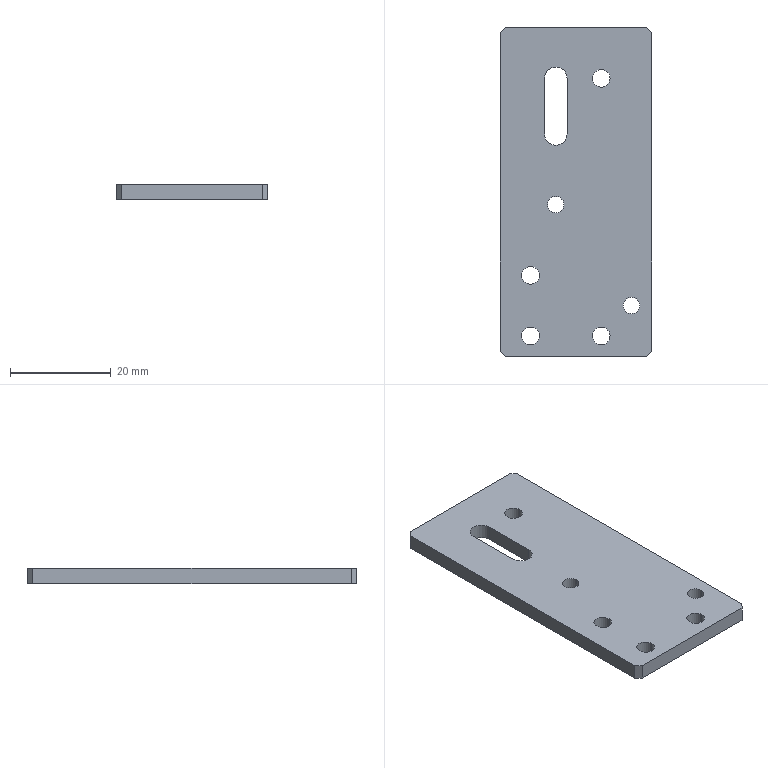Part | SolidWorks | features BaseBody 1 | 1 solid | 26 faces | box 30 x 65 x 3 mm | volume 5483 mm3 | cylinder 14 | plane 12 | commonest cylinder face diameters 3.5 x8 3.242 x4 4.5 x2
STEP:
#1=CARTESIAN_POINT('',(-39.084,79.458,0.));
#2=VERTEX_POINT('',#1);
#3=CARTESIAN_POINT('',(-42.584,79.458,0.));
#4=VERTEX_POINT('',#3);
#5=CARTESIAN_POINT('',(-40.834,79.458,0.));
#6=DIRECTION('',(0.,0.,-1.));
#7=DIRECTION('',(1.,0.,0.));
#8=AXIS2_PLACEMENT_3D('',#5,#6,#7);
#9=CIRCLE('',#8,1.75);
#10=EDGE_CURVE('',#2,#4,#9,.T.);
#11=ORIENTED_EDGE('',*,*,#10,.T.);
#12=CARTESIAN_POINT('',(-42.584,79.458,3.));
#13=VERTEX_POINT('',#12);
#14=CARTESIAN_POINT('',(-42.584,79.458,-68.652));
#15=DIRECTION('',(0.,0.,1.));
#16=VECTOR('',#15,1000.);
#17=LINE('',#14,#16);
#18=EDGE_CURVE('',#4,#13,#17,.T.);
#19=ORIENTED_EDGE('',*,*,#18,.T.);
#20=CARTESIAN_POINT('',(-39.084,79.458,3.));
#21=VERTEX_POINT('',#20);
#22=CARTESIAN_POINT('',(-40.834,79.458,3.));
#23=DIRECTION('',(0.,0.,-1.));
#24=DIRECTION('',(1.,0.,0.));
#25=AXIS2_PLACEMENT_3D('',#22,#23,#24);
#26=CIRCLE('',#25,1.75);
#27=EDGE_CURVE('',#21,#13,#26,.T.);
#28=ORIENTED_EDGE('',*,*,#27,.F.);
#29=CARTESIAN_POINT('',(-39.084,79.458,-68.652));
#30=DIRECTION('',(0.,0.,1.));
#31=VECTOR('',#30,1000.);
#32=LINE('',#29,#31);
#33=EDGE_CURVE('',#2,#21,#32,.T.);
#34=ORIENTED_EDGE('',*,*,#33,.F.);
#35=EDGE_LOOP('',(#11,#19,#28,#34));
#36=FACE_OUTER_BOUND('',#35,.T.);
#37=CARTESIAN_POINT('',(-40.834,79.458,-68.652));
#38=DIRECTION('',(0.,0.,1.));
#39=DIRECTION('',(1.,0.,0.));
#40=AXIS2_PLACEMENT_3D('',#37,#38,#39);
#41=CYLINDRICAL_SURFACE('',#40,1.75);
#42=ADVANCED_FACE('',(#36),#41,.F.);
#43=CARTESIAN_POINT('',(-53.084,79.458,0.));
#44=VERTEX_POINT('',#43);
#45=CARTESIAN_POINT('',(-56.584,79.458,0.));
#46=VERTEX_POINT('',#45);
#47=CARTESIAN_POINT('',(-54.834,79.458,0.));
#48=DIRECTION('',(0.,0.,-1.));
#49=DIRECTION('',(1.,0.,0.));
#50=AXIS2_PLACEMENT_3D('',#47,#48,#49);
#51=CIRCLE('',#50,1.75);
#52=EDGE_CURVE('',#44,#46,#51,.T.);
#53=ORIENTED_EDGE('',*,*,#52,.T.);
#54=CARTESIAN_POINT('',(-56.584,79.458,3.));
#55=VERTEX_POINT('',#54);
#56=CARTESIAN_POINT('',(-56.584,79.458,-68.652));
#57=DIRECTION('',(0.,0.,1.));
#58=VECTOR('',#57,1000.);
#59=LINE('',#56,#58);
#60=EDGE_CURVE('',#46,#55,#59,.T.);
#61=ORIENTED_EDGE('',*,*,#60,.T.);
#62=CARTESIAN_POINT('',(-53.084,79.458,3.));
#63=VERTEX_POINT('',#62);
#64=CARTESIAN_POINT('',(-54.834,79.458,3.));
#65=DIRECTION('',(0.,0.,-1.));
#66=DIRECTION('',(1.,0.,0.));
#67=AXIS2_PLACEMENT_3D('',#64,#65,#66);
#68=CIRCLE('',#67,1.75);
#69=EDGE_CURVE('',#63,#55,#68,.T.);
#70=ORIENTED_EDGE('',*,*,#69,.F.);
#71=CARTESIAN_POINT('',(-53.084,79.458,-68.652));
#72=DIRECTION('',(0.,0.,1.));
#73=VECTOR('',#72,1000.);
#74=LINE('',#71,#73);
#75=EDGE_CURVE('',#44,#63,#74,.T.);
#76=ORIENTED_EDGE('',*,*,#75,.F.);
#77=EDGE_LOOP('',(#53,#61,#70,#76));
#78=FACE_OUTER_BOUND('',#77,.T.);
#79=CARTESIAN_POINT('',(-54.834,79.458,-68.652));
#80=DIRECTION('',(0.,0.,1.));
#81=DIRECTION('',(1.,0.,0.));
#82=AXIS2_PLACEMENT_3D('',#79,#80,#81);
#83=CYLINDRICAL_SURFACE('',#82,1.75);
#84=ADVANCED_FACE('',(#78),#83,.F.);
#85=CARTESIAN_POINT('',(-53.084,91.458,0.));
#86=VERTEX_POINT('',#85);
#87=CARTESIAN_POINT('',(-56.584,91.458,0.));
#88=VERTEX_POINT('',#87);
#89=CARTESIAN_POINT('',(-54.834,91.458,0.));
#90=DIRECTION('',(0.,0.,-1.));
#91=DIRECTION('',(1.,0.,0.));
#92=AXIS2_PLACEMENT_3D('',#89,#90,#91);
#93=CIRCLE('',#92,1.75);
#94=EDGE_CURVE('',#86,#88,#93,.T.);
#95=ORIENTED_EDGE('',*,*,#94,.T.);
#96=CARTESIAN_POINT('',(-56.584,91.458,3.));
#97=VERTEX_POINT('',#96);
#98=CARTESIAN_POINT('',(-56.584,91.458,-68.652));
#99=DIRECTION('',(0.,0.,1.));
#100=VECTOR('',#99,1000.);
#101=LINE('',#98,#100);
#102=EDGE_CURVE('',#88,#97,#101,.T.);
#103=ORIENTED_EDGE('',*,*,#102,.T.);
#104=CARTESIAN_POINT('',(-53.084,91.458,3.));
#105=VERTEX_POINT('',#104);
#106=CARTESIAN_POINT('',(-54.834,91.458,3.));
#107=DIRECTION('',(0.,0.,-1.));
#108=DIRECTION('',(1.,0.,0.));
#109=AXIS2_PLACEMENT_3D('',#106,#107,#108);
#110=CIRCLE('',#109,1.75);
#111=EDGE_CURVE('',#105,#97,#110,.T.);
#112=ORIENTED_EDGE('',*,*,#111,.F.);
#113=CARTESIAN_POINT('',(-53.084,91.458,-68.652));
#114=DIRECTION('',(0.,0.,1.));
#115=VECTOR('',#114,1000.);
#116=LINE('',#113,#115);
#117=EDGE_CURVE('',#86,#105,#116,.T.);
#118=ORIENTED_EDGE('',*,*,#117,.F.);
#119=EDGE_LOOP('',(#95,#103,#112,#118));
#120=FACE_OUTER_BOUND('',#119,.T.);
#121=CARTESIAN_POINT('',(-54.834,91.458,-68.652));
#122=DIRECTION('',(0.,0.,1.));
#123=DIRECTION('',(1.,0.,0.));
#124=AXIS2_PLACEMENT_3D('',#121,#122,#123);
#125=CYLINDRICAL_SURFACE('',#124,1.75);
#126=ADVANCED_FACE('',(#120),#125,.F.);
#127=CARTESIAN_POINT('',(-39.084,130.458,0.));
#128=VERTEX_POINT('',#127);
#129=CARTESIAN_POINT('',(-42.584,130.458,0.));
#130=VERTEX_POINT('',#129);
#131=CARTESIAN_POINT('',(-40.834,130.458,0.));
#132=DIRECTION('',(0.,0.,-1.));
#133=DIRECTION('',(1.,0.,0.));
#134=AXIS2_PLACEMENT_3D('',#131,#132,#133);
#135=CIRCLE('',#134,1.75);
#136=EDGE_CURVE('',#128,#130,#135,.T.);
#137=ORIENTED_EDGE('',*,*,#136,.T.);
#138=CARTESIAN_POINT('',(-42.584,130.458,3.));
#139=VERTEX_POINT('',#138);
#140=CARTESIAN_POINT('',(-42.584,130.458,-68.652));
#141=DIRECTION('',(0.,0.,1.));
#142=VECTOR('',#141,1000.);
#143=LINE('',#140,#142);
#144=EDGE_CURVE('',#130,#139,#143,.T.);
#145=ORIENTED_EDGE('',*,*,#144,.T.);
#146=CARTESIAN_POINT('',(-39.084,130.458,3.));
#147=VERTEX_POINT('',#146);
#148=CARTESIAN_POINT('',(-40.834,130.458,3.));
#149=DIRECTION('',(0.,0.,-1.));
#150=DIRECTION('',(1.,0.,0.));
#151=AXIS2_PLACEMENT_3D('',#148,#149,#150);
#152=CIRCLE('',#151,1.75);
#153=EDGE_CURVE('',#147,#139,#152,.T.);
#154=ORIENTED_EDGE('',*,*,#153,.F.);
#155=CARTESIAN_POINT('',(-39.084,130.458,-68.652));
#156=DIRECTION('',(0.,0.,1.));
#157=VECTOR('',#156,1000.);
#158=LINE('',#155,#157);
#159=EDGE_CURVE('',#128,#147,#158,.T.);
#160=ORIENTED_EDGE('',*,*,#159,.F.);
#161=EDGE_LOOP('',(#137,#145,#154,#160));
#162=FACE_OUTER_BOUND('',#161,.T.);
#163=CARTESIAN_POINT('',(-40.834,130.458,-68.652));
#164=DIRECTION('',(0.,0.,1.));
#165=DIRECTION('',(1.,0.,0.));
#166=AXIS2_PLACEMENT_3D('',#163,#164,#165);
#167=CYLINDRICAL_SURFACE('',#166,1.75);
#168=ADVANCED_FACE('',(#162),#167,.F.);
#169=CARTESIAN_POINT('',(-33.213,85.458,0.));
#170=VERTEX_POINT('',#169);
#171=CARTESIAN_POINT('',(-36.455,85.458,0.));
#172=VERTEX_POINT('',#171);
#173=CARTESIAN_POINT('',(-34.834,85.458,0.));
#174=DIRECTION('',(0.,0.,-1.));
#175=DIRECTION('',(1.,0.,0.));
#176=AXIS2_PLACEMENT_3D('',#173,#174,#175);
#177=CIRCLE('',#176,1.621);
#178=EDGE_CURVE('',#170,#172,#177,.T.);
#179=ORIENTED_EDGE('',*,*,#178,.T.);
#180=CARTESIAN_POINT('',(-36.455,85.458,3.));
#181=VERTEX_POINT('',#180);
#182=CARTESIAN_POINT('',(-36.455,85.458,-68.652));
#183=DIRECTION('',(0.,0.,1.));
#184=VECTOR('',#183,1000.);
#185=LINE('',#182,#184);
#186=EDGE_CURVE('',#172,#181,#185,.T.);
#187=ORIENTED_EDGE('',*,*,#186,.T.);
#188=CARTESIAN_POINT('',(-33.213,85.458,3.));
#189=VERTEX_POINT('',#188);
#190=CARTESIAN_POINT('',(-34.834,85.458,3.));
#191=DIRECTION('',(0.,0.,-1.));
#192=DIRECTION('',(1.,0.,0.));
#193=AXIS2_PLACEMENT_3D('',#190,#191,#192);
#194=CIRCLE('',#193,1.621);
#195=EDGE_CURVE('',#189,#181,#194,.T.);
#196=ORIENTED_EDGE('',*,*,#195,.F.);
#197=CARTESIAN_POINT('',(-33.213,85.458,-68.652));
#198=DIRECTION('',(0.,0.,1.));
#199=VECTOR('',#198,1000.);
#200=LINE('',#197,#199);
#201=EDGE_CURVE('',#170,#189,#200,.T.);
#202=ORIENTED_EDGE('',*,*,#201,.F.);
#203=EDGE_LOOP('',(#179,#187,#196,#202));
#204=FACE_OUTER_BOUND('',#203,.T.);
#205=CARTESIAN_POINT('',(-34.834,85.458,-68.652));
#206=DIRECTION('',(0.,0.,1.));
#207=DIRECTION('',(1.,0.,0.));
#208=AXIS2_PLACEMENT_3D('',#205,#206,#207);
#209=CYLINDRICAL_SURFACE('',#208,1.621);
#210=ADVANCED_FACE('',(#204),#209,.F.);
#211=CARTESIAN_POINT('',(-48.213,105.458,0.));
#212=VERTEX_POINT('',#211);
#213=CARTESIAN_POINT('',(-51.455,105.458,0.));
#214=VERTEX_POINT('',#213);
#215=CARTESIAN_POINT('',(-49.834,105.458,0.));
#216=DIRECTION('',(0.,0.,-1.));
#217=DIRECTION('',(1.,0.,0.));
#218=AXIS2_PLACEMENT_3D('',#215,#216,#217);
#219=CIRCLE('',#218,1.621);
#220=EDGE_CURVE('',#212,#214,#219,.T.);
#221=ORIENTED_EDGE('',*,*,#220,.T.);
#222=CARTESIAN_POINT('',(-51.455,105.458,3.));
#223=VERTEX_POINT('',#222);
#224=CARTESIAN_POINT('',(-51.455,105.458,-68.652));
#225=DIRECTION('',(0.,0.,1.));
#226=VECTOR('',#225,1000.);
#227=LINE('',#224,#226);
#228=EDGE_CURVE('',#214,#223,#227,.T.);
#229=ORIENTED_EDGE('',*,*,#228,.T.);
#230=CARTESIAN_POINT('',(-48.213,105.458,3.));
#231=VERTEX_POINT('',#230);
#232=CARTESIAN_POINT('',(-49.834,105.458,3.));
#233=DIRECTION('',(0.,0.,-1.));
#234=DIRECTION('',(1.,0.,0.));
#235=AXIS2_PLACEMENT_3D('',#232,#233,#234);
#236=CIRCLE('',#235,1.621);
#237=EDGE_CURVE('',#231,#223,#236,.T.);
#238=ORIENTED_EDGE('',*,*,#237,.F.);
#239=CARTESIAN_POINT('',(-48.213,105.458,-68.652));
#240=DIRECTION('',(0.,0.,1.));
#241=VECTOR('',#240,1000.);
#242=LINE('',#239,#241);
#243=EDGE_CURVE('',#212,#231,#242,.T.);
#244=ORIENTED_EDGE('',*,*,#243,.F.);
#245=EDGE_LOOP('',(#221,#229,#238,#244));
#246=FACE_OUTER_BOUND('',#245,.T.);
#247=CARTESIAN_POINT('',(-49.834,105.458,-68.652));
#248=DIRECTION('',(0.,0.,1.));
#249=DIRECTION('',(1.,0.,0.));
#250=AXIS2_PLACEMENT_3D('',#247,#248,#249);
#251=CYLINDRICAL_SURFACE('',#250,1.621);
#252=ADVANCED_FACE('',(#246),#251,.F.);
#253=ORIENTED_EDGE('',*,*,#10,.F.);
#254=CARTESIAN_POINT('',(-40.834,79.458,0.));
#255=DIRECTION('',(0.,0.,-1.));
#256=DIRECTION('',(1.,0.,0.));
#257=AXIS2_PLACEMENT_3D('',#254,#255,#256);
#258=CIRCLE('',#257,1.75);
#259=EDGE_CURVE('',#4,#2,#258,.T.);
#260=ORIENTED_EDGE('',*,*,#259,.F.);
#261=EDGE_LOOP('',(#253,#260));
#262=FACE_BOUND('',#261,.T.);
#263=ORIENTED_EDGE('',*,*,#52,.F.);
#264=CARTESIAN_POINT('',(-54.834,79.458,0.));
#265=DIRECTION('',(0.,0.,-1.));
#266=DIRECTION('',(1.,0.,0.));
#267=AXIS2_PLACEMENT_3D('',#264,#265,#266);
#268=CIRCLE('',#267,1.75);
#269=EDGE_CURVE('',#46,#44,#268,.T.);
#270=ORIENTED_EDGE('',*,*,#269,.F.);
#271=EDGE_LOOP('',(#263,#270));
#272=FACE_BOUND('',#271,.T.);
#273=ORIENTED_EDGE('',*,*,#94,.F.);
#274=CARTESIAN_POINT('',(-54.834,91.458,0.));
#275=DIRECTION('',(0.,0.,-1.));
#276=DIRECTION('',(1.,0.,0.));
#277=AXIS2_PLACEMENT_3D('',#274,#275,#276);
#278=CIRCLE('',#277,1.75);
#279=EDGE_CURVE('',#88,#86,#278,.T.);
#280=ORIENTED_EDGE('',*,*,#279,.F.);
#281=EDGE_LOOP('',(#273,#280));
#282=FACE_BOUND('',#281,.T.);
#283=ORIENTED_EDGE('',*,*,#136,.F.);
#284=CARTESIAN_POINT('',(-40.834,130.458,0.));
#285=DIRECTION('',(0.,0.,-1.));
#286=DIRECTION('',(1.,0.,0.));
#287=AXIS2_PLACEMENT_3D('',#284,#285,#286);
#288=CIRCLE('',#287,1.75);
#289=EDGE_CURVE('',#130,#128,#288,.T.);
#290=ORIENTED_EDGE('',*,*,#289,.F.);
#291=EDGE_LOOP('',(#283,#290));
#292=FACE_BOUND('',#291,.T.);
#293=ORIENTED_EDGE('',*,*,#178,.F.);
#294=CARTESIAN_POINT('',(-34.834,85.458,0.));
#295=DIRECTION('',(0.,0.,-1.));
#296=DIRECTION('',(1.,0.,0.));
#297=AXIS2_PLACEMENT_3D('',#294,#295,#296);
#298=CIRCLE('',#297,1.621);
#299=EDGE_CURVE('',#172,#170,#298,.T.);
#300=ORIENTED_EDGE('',*,*,#299,.F.);
#301=EDGE_LOOP('',(#293,#300));
#302=FACE_BOUND('',#301,.T.);
#303=ORIENTED_EDGE('',*,*,#220,.F.);
#304=CARTESIAN_POINT('',(-49.834,105.458,0.));
#305=DIRECTION('',(0.,0.,-1.));
#306=DIRECTION('',(1.,0.,0.));
#307=AXIS2_PLACEMENT_3D('',#304,#305,#306);
#308=CIRCLE('',#307,1.621);
#309=EDGE_CURVE('',#214,#212,#308,.T.);
#310=ORIENTED_EDGE('',*,*,#309,.F.);
#311=EDGE_LOOP('',(#303,#310));
#312=FACE_BOUND('',#311,.T.);
#313=CARTESIAN_POINT('',(-47.584,119.458,0.));
#314=VERTEX_POINT('',#313);
#315=CARTESIAN_POINT('',(-52.084,119.458,0.));
#316=VERTEX_POINT('',#315);
#317=CARTESIAN_POINT('',(-49.834,119.458,0.));
#318=DIRECTION('',(0.,0.,-1.));
#319=DIRECTION('',(-1.,0.,0.));
#320=AXIS2_PLACEMENT_3D('',#317,#318,#319);
#321=CIRCLE('',#320,2.25);
#322=EDGE_CURVE('',#314,#316,#321,.T.);
#323=ORIENTED_EDGE('',*,*,#322,.F.);
#324=CARTESIAN_POINT('',(-47.584,130.458,0.));
#325=VERTEX_POINT('',#324);
#326=CARTESIAN_POINT('',(-47.584,107.958,0.));
#327=DIRECTION('',(0.,-1.,0.));
#328=VECTOR('',#327,1000.);
#329=LINE('',#326,#328);
#330=EDGE_CURVE('',#325,#314,#329,.T.);
#331=ORIENTED_EDGE('',*,*,#330,.F.);
#332=CARTESIAN_POINT('',(-52.084,130.458,0.));
#333=VERTEX_POINT('',#332);
#334=CARTESIAN_POINT('',(-49.834,130.458,0.));
#335=DIRECTION('',(0.,0.,-1.));
#336=DIRECTION('',(-1.,0.,0.));
#337=AXIS2_PLACEMENT_3D('',#334,#335,#336);
#338=CIRCLE('',#337,2.25);
#339=EDGE_CURVE('',#333,#325,#338,.T.);
#340=ORIENTED_EDGE('',*,*,#339,.F.);
#341=CARTESIAN_POINT('',(-52.084,107.958,0.));
#342=DIRECTION('',(0.,1.,0.));
#343=VECTOR('',#342,1000.);
#344=LINE('',#341,#343);
#345=EDGE_CURVE('',#316,#333,#344,.T.);
#346=ORIENTED_EDGE('',*,*,#345,.F.);
#347=EDGE_LOOP('',(#323,#331,#340,#346));
#348=FACE_BOUND('',#347,.T.);
#349=CARTESIAN_POINT('',(-60.834,139.458,0.));
#350=VERTEX_POINT('',#349);
#351=CARTESIAN_POINT('',(-60.834,76.458,0.));
#352=VERTEX_POINT('',#351);
#353=CARTESIAN_POINT('',(-60.834,107.958,0.));
#354=DIRECTION('',(0.,-1.,0.));
#355=VECTOR('',#354,1000.);
#356=LINE('',#353,#355);
#357=EDGE_CURVE('',#350,#352,#356,.T.);
#358=ORIENTED_EDGE('',*,*,#357,.F.);
#359=CARTESIAN_POINT('',(-59.834,140.458,0.));
#360=VERTEX_POINT('',#359);
#361=CARTESIAN_POINT('',(-60.334,139.958,0.));
#362=DIRECTION('',(-0.7071,-0.7071,0.));
#363=VECTOR('',#362,1000.);
#364=LINE('',#361,#363);
#365=EDGE_CURVE('',#360,#350,#364,.T.);
#366=ORIENTED_EDGE('',*,*,#365,.F.);
#367=CARTESIAN_POINT('',(-31.834,140.458,0.));
#368=VERTEX_POINT('',#367);
#369=CARTESIAN_POINT('',(-45.834,140.458,0.));
#370=DIRECTION('',(-1.,0.,0.));
#371=VECTOR('',#370,1000.);
#372=LINE('',#369,#371);
#373=EDGE_CURVE('',#368,#360,#372,.T.);
#374=ORIENTED_EDGE('',*,*,#373,.F.);
#375=CARTESIAN_POINT('',(-30.834,139.458,0.));
#376=VERTEX_POINT('',#375);
#377=CARTESIAN_POINT('',(-31.334,139.958,0.));
#378=DIRECTION('',(-0.7071,0.7071,0.));
#379=VECTOR('',#378,1000.);
#380=LINE('',#377,#379);
#381=EDGE_CURVE('',#376,#368,#380,.T.);
#382=ORIENTED_EDGE('',*,*,#381,.F.);
#383=CARTESIAN_POINT('',(-30.834,76.458,0.));
#384=VERTEX_POINT('',#383);
#385=CARTESIAN_POINT('',(-30.834,107.958,0.));
#386=DIRECTION('',(0.,1.,0.));
#387=VECTOR('',#386,1000.);
#388=LINE('',#385,#387);
#389=EDGE_CURVE('',#384,#376,#388,.T.);
#390=ORIENTED_EDGE('',*,*,#389,.F.);
#391=CARTESIAN_POINT('',(-31.834,75.458,0.));
#392=VERTEX_POINT('',#391);
#393=CARTESIAN_POINT('',(-31.334,75.958,0.));
#394=DIRECTION('',(0.7071,0.7071,0.));
#395=VECTOR('',#394,1000.);
#396=LINE('',#393,#395);
#397=EDGE_CURVE('',#392,#384,#396,.T.);
#398=ORIENTED_EDGE('',*,*,#397,.F.);
#399=CARTESIAN_POINT('',(-59.834,75.458,0.));
#400=VERTEX_POINT('',#399);
#401=CARTESIAN_POINT('',(-45.834,75.458,0.));
#402=DIRECTION('',(1.,0.,0.));
#403=VECTOR('',#402,1000.);
#404=LINE('',#401,#403);
#405=EDGE_CURVE('',#400,#392,#404,.T.);
#406=ORIENTED_EDGE('',*,*,#405,.F.);
#407=CARTESIAN_POINT('',(-60.334,75.958,0.));
#408=DIRECTION('',(0.7071,-0.7071,0.));
#409=VECTOR('',#408,1000.);
#410=LINE('',#407,#409);
#411=EDGE_CURVE('',#352,#400,#410,.T.);
#412=ORIENTED_EDGE('',*,*,#411,.F.);
#413=EDGE_LOOP('',(#358,#366,#374,#382,#390,#398,#406,#412));
#414=FACE_OUTER_BOUND('',#413,.T.);
#415=CARTESIAN_POINT('',(-45.834,107.958,0.));
#416=DIRECTION('',(0.,0.,1.));
#417=DIRECTION('',(1.,0.,0.));
#418=AXIS2_PLACEMENT_3D('',#415,#416,#417);
#419=PLANE('',#418);
#420=ADVANCED_FACE('',(#262,#272,#282,#292,#302,#312,#348,#414),#419,.F.);
#421=ORIENTED_EDGE('',*,*,#18,.F.);
#422=ORIENTED_EDGE('',*,*,#259,.T.);
#423=ORIENTED_EDGE('',*,*,#33,.T.);
#424=CARTESIAN_POINT('',(-40.834,79.458,3.));
#425=DIRECTION('',(0.,0.,-1.));
#426=DIRECTION('',(1.,0.,0.));
#427=AXIS2_PLACEMENT_3D('',#424,#425,#426);
#428=CIRCLE('',#427,1.75);
#429=EDGE_CURVE('',#13,#21,#428,.T.);
#430=ORIENTED_EDGE('',*,*,#429,.F.);
#431=EDGE_LOOP('',(#421,#422,#423,#430));
#432=FACE_OUTER_BOUND('',#431,.T.);
#433=CARTESIAN_POINT('',(-40.834,79.458,-68.652));
#434=DIRECTION('',(0.,0.,1.));
#435=DIRECTION('',(1.,0.,0.));
#436=AXIS2_PLACEMENT_3D('',#433,#434,#435);
#437=CYLINDRICAL_SURFACE('',#436,1.75);
#438=ADVANCED_FACE('',(#432),#437,.F.);
#439=ORIENTED_EDGE('',*,*,#60,.F.);
#440=ORIENTED_EDGE('',*,*,#269,.T.);
#441=ORIENTED_EDGE('',*,*,#75,.T.);
#442=CARTESIAN_POINT('',(-54.834,79.458,3.));
#443=DIRECTION('',(0.,0.,-1.));
#444=DIRECTION('',(1.,0.,0.));
#445=AXIS2_PLACEMENT_3D('',#442,#443,#444);
#446=CIRCLE('',#445,1.75);
#447=EDGE_CURVE('',#55,#63,#446,.T.);
#448=ORIENTED_EDGE('',*,*,#447,.F.);
#449=EDGE_LOOP('',(#439,#440,#441,#448));
#450=FACE_OUTER_BOUND('',#449,.T.);
#451=CARTESIAN_POINT('',(-54.834,79.458,-68.652));
#452=DIRECTION('',(0.,0.,1.));
#453=DIRECTION('',(1.,0.,0.));
#454=AXIS2_PLACEMENT_3D('',#451,#452,#453);
#455=CYLINDRICAL_SURFACE('',#454,1.75);
#456=ADVANCED_FACE('',(#450),#455,.F.);
#457=ORIENTED_EDGE('',*,*,#102,.F.);
#458=ORIENTED_EDGE('',*,*,#279,.T.);
#459=ORIENTED_EDGE('',*,*,#117,.T.);
#460=CARTESIAN_POINT('',(-54.834,91.458,3.));
#461=DIRECTION('',(0.,0.,-1.));
#462=DIRECTION('',(1.,0.,0.));
#463=AXIS2_PLACEMENT_3D('',#460,#461,#462);
#464=CIRCLE('',#463,1.75);
#465=EDGE_CURVE('',#97,#105,#464,.T.);
#466=ORIENTED_EDGE('',*,*,#465,.F.);
#467=EDGE_LOOP('',(#457,#458,#459,#466));
#468=FACE_OUTER_BOUND('',#467,.T.);
#469=CARTESIAN_POINT('',(-54.834,91.458,-68.652));
#470=DIRECTION('',(0.,0.,1.));
#471=DIRECTION('',(1.,0.,0.));
#472=AXIS2_PLACEMENT_3D('',#469,#470,#471);
#473=CYLINDRICAL_SURFACE('',#472,1.75);
#474=ADVANCED_FACE('',(#468),#473,.F.);
#475=ORIENTED_EDGE('',*,*,#144,.F.);
#476=ORIENTED_EDGE('',*,*,#289,.T.);
#477=ORIENTED_EDGE('',*,*,#159,.T.);
#478=CARTESIAN_POINT('',(-40.834,130.458,3.));
#479=DIRECTION('',(0.,0.,-1.));
#480=DIRECTION('',(1.,0.,0.));
#481=AXIS2_PLACEMENT_3D('',#478,#479,#480);
#482=CIRCLE('',#481,1.75);
#483=EDGE_CURVE('',#139,#147,#482,.T.);
#484=ORIENTED_EDGE('',*,*,#483,.F.);
#485=EDGE_LOOP('',(#475,#476,#477,#484));
#486=FACE_OUTER_BOUND('',#485,.T.);
#487=CARTESIAN_POINT('',(-40.834,130.458,-68.652));
#488=DIRECTION('',(0.,0.,1.));
#489=DIRECTION('',(1.,0.,0.));
#490=AXIS2_PLACEMENT_3D('',#487,#488,#489);
#491=CYLINDRICAL_SURFACE('',#490,1.75);
#492=ADVANCED_FACE('',(#486),#491,.F.);
#493=ORIENTED_EDGE('',*,*,#186,.F.);
#494=ORIENTED_EDGE('',*,*,#299,.T.);
#495=ORIENTED_EDGE('',*,*,#201,.T.);
#496=CARTESIAN_POINT('',(-34.834,85.458,3.));
#497=DIRECTION('',(0.,0.,-1.));
#498=DIRECTION('',(1.,0.,0.));
#499=AXIS2_PLACEMENT_3D('',#496,#497,#498);
#500=CIRCLE('',#499,1.621);
#501=EDGE_CURVE('',#181,#189,#500,.T.);
#502=ORIENTED_EDGE('',*,*,#501,.F.);
#503=EDGE_LOOP('',(#493,#494,#495,#502));
#504=FACE_OUTER_BOUND('',#503,.T.);
#505=CARTESIAN_POINT('',(-34.834,85.458,-68.652));
#506=DIRECTION('',(0.,0.,1.));
#507=DIRECTION('',(1.,0.,0.));
#508=AXIS2_PLACEMENT_3D('',#505,#506,#507);
#509=CYLINDRICAL_SURFACE('',#508,1.621);
#510=ADVANCED_FACE('',(#504),#509,.F.);
#511=ORIENTED_EDGE('',*,*,#228,.F.);
#512=ORIENTED_EDGE('',*,*,#309,.T.);
#513=ORIENTED_EDGE('',*,*,#243,.T.);
#514=CARTESIAN_POINT('',(-49.834,105.458,3.));
#515=DIRECTION('',(0.,0.,-1.));
#516=DIRECTION('',(1.,0.,0.));
#517=AXIS2_PLACEMENT_3D('',#514,#515,#516);
#518=CIRCLE('',#517,1.621);
#519=EDGE_CURVE('',#223,#231,#518,.T.);
#520=ORIENTED_EDGE('',*,*,#519,.F.);
#521=EDGE_LOOP('',(#511,#512,#513,#520));
#522=FACE_OUTER_BOUND('',#521,.T.);
#523=CARTESIAN_POINT('',(-49.834,105.458,-68.652));
#524=DIRECTION('',(0.,0.,1.));
#525=DIRECTION('',(1.,0.,0.));
#526=AXIS2_PLACEMENT_3D('',#523,#524,#525);
#527=CYLINDRICAL_SURFACE('',#526,1.621);
#528=ADVANCED_FACE('',(#522),#527,.F.);
#529=CARTESIAN_POINT('',(-52.084,130.458,3.));
#530=VERTEX_POINT('',#529);
#531=CARTESIAN_POINT('',(-52.084,130.458,3.));
#532=DIRECTION('',(0.,0.,-1.));
#533=VECTOR('',#532,1000.);
#534=LINE('',#531,#533);
#535=EDGE_CURVE('',#530,#333,#534,.T.);
#536=ORIENTED_EDGE('',*,*,#535,.F.);
#537=CARTESIAN_POINT('',(-52.084,119.458,3.));
#538=VERTEX_POINT('',#537);
#539=CARTESIAN_POINT('',(-52.084,130.458,3.));
#540=DIRECTION('',(0.,1.,0.));
#541=VECTOR('',#540,1000.);
#542=LINE('',#539,#541);
#543=EDGE_CURVE('',#538,#530,#542,.T.);
#544=ORIENTED_EDGE('',*,*,#543,.F.);
#545=CARTESIAN_POINT('',(-52.084,119.458,3.));
#546=DIRECTION('',(0.,0.,1.));
#547=VECTOR('',#546,1000.);
#548=LINE('',#545,#547);
#549=EDGE_CURVE('',#316,#538,#548,.T.);
#550=ORIENTED_EDGE('',*,*,#549,.F.);
#551=ORIENTED_EDGE('',*,*,#345,.T.);
#552=EDGE_LOOP('',(#536,#544,#550,#551));
#553=FACE_OUTER_BOUND('',#552,.T.);
#554=CARTESIAN_POINT('',(-52.084,130.458,3.));
#555=DIRECTION('',(-1.,0.,0.));
#556=DIRECTION('',(0.,0.,1.));
#557=AXIS2_PLACEMENT_3D('',#554,#555,#556);
#558=PLANE('',#557);
#559=ADVANCED_FACE('',(#553),#558,.F.);
#560=ORIENTED_EDGE('',*,*,#549,.T.);
#561=CARTESIAN_POINT('',(-47.584,119.458,3.));
#562=VERTEX_POINT('',#561);
#563=CARTESIAN_POINT('',(-49.834,119.458,3.));
#564=DIRECTION('',(0.,0.,-1.));
#565=DIRECTION('',(-1.,0.,0.));
#566=AXIS2_PLACEMENT_3D('',#563,#564,#565);
#567=CIRCLE('',#566,2.25);
#568=EDGE_CURVE('',#562,#538,#567,.T.);
#569=ORIENTED_EDGE('',*,*,#568,.F.);
#570=CARTESIAN_POINT('',(-47.584,119.458,3.));
#571=DIRECTION('',(0.,0.,1.));
#572=VECTOR('',#571,1000.);
#573=LINE('',#570,#572);
#574=EDGE_CURVE('',#314,#562,#573,.T.);
#575=ORIENTED_EDGE('',*,*,#574,.F.);
#576=ORIENTED_EDGE('',*,*,#322,.T.);
#577=EDGE_LOOP('',(#560,#569,#575,#576));
#578=FACE_OUTER_BOUND('',#577,.T.);
#579=CARTESIAN_POINT('',(-49.834,119.458,3.));
#580=DIRECTION('',(0.,0.,-1.));
#581=DIRECTION('',(-1.,0.,0.));
#582=AXIS2_PLACEMENT_3D('',#579,#580,#581);
#583=CYLINDRICAL_SURFACE('',#582,2.25);
#584=ADVANCED_FACE('',(#578),#583,.F.);
#585=ORIENTED_EDGE('',*,*,#574,.T.);
#586=CARTESIAN_POINT('',(-47.584,130.458,3.));
#587=VERTEX_POINT('',#586);
#588=CARTESIAN_POINT('',(-47.584,119.458,3.));
#589=DIRECTION('',(0.,-1.,0.));
#590=VECTOR('',#589,1000.);
#591=LINE('',#588,#590);
#592=EDGE_CURVE('',#587,#562,#591,.T.);
#593=ORIENTED_EDGE('',*,*,#592,.F.);
#594=CARTESIAN_POINT('',(-47.584,130.458,3.));
#595=DIRECTION('',(0.,0.,1.));
#596=VECTOR('',#595,1000.);
#597=LINE('',#594,#596);
#598=EDGE_CURVE('',#325,#587,#597,.T.);
#599=ORIENTED_EDGE('',*,*,#598,.F.);
#600=ORIENTED_EDGE('',*,*,#330,.T.);
#601=EDGE_LOOP('',(#585,#593,#599,#600));
#602=FACE_OUTER_BOUND('',#601,.T.);
#603=CARTESIAN_POINT('',(-47.584,119.458,3.));
#604=DIRECTION('',(1.,0.,0.));
#605=DIRECTION('',(0.,0.,-1.));
#606=AXIS2_PLACEMENT_3D('',#603,#604,#605);
#607=PLANE('',#606);
#608=ADVANCED_FACE('',(#602),#607,.F.);
#609=ORIENTED_EDGE('',*,*,#598,.T.);
#610=CARTESIAN_POINT('',(-49.834,130.458,3.));
#611=DIRECTION('',(0.,0.,-1.));
#612=DIRECTION('',(-1.,0.,0.));
#613=AXIS2_PLACEMENT_3D('',#610,#611,#612);
#614=CIRCLE('',#613,2.25);
#615=EDGE_CURVE('',#530,#587,#614,.T.);
#616=ORIENTED_EDGE('',*,*,#615,.F.);
#617=ORIENTED_EDGE('',*,*,#535,.T.);
#618=ORIENTED_EDGE('',*,*,#339,.T.);
#619=EDGE_LOOP('',(#609,#616,#617,#618));
#620=FACE_OUTER_BOUND('',#619,.T.);
#621=CARTESIAN_POINT('',(-49.834,130.458,3.));
#622=DIRECTION('',(0.,0.,-1.));
#623=DIRECTION('',(-1.,0.,0.));
#624=AXIS2_PLACEMENT_3D('',#621,#622,#623);
#625=CYLINDRICAL_SURFACE('',#624,2.25);
#626=ADVANCED_FACE('',(#620),#625,.F.);
#627=CARTESIAN_POINT('',(-60.834,139.458,3.));
#628=VERTEX_POINT('',#627);
#629=CARTESIAN_POINT('',(-60.834,139.458,0.));
#630=DIRECTION('',(0.,0.,-1.));
#631=VECTOR('',#630,1000.);
#632=LINE('',#629,#631);
#633=EDGE_CURVE('',#628,#350,#632,.T.);
#634=ORIENTED_EDGE('',*,*,#633,.T.);
#635=ORIENTED_EDGE('',*,*,#357,.T.);
#636=CARTESIAN_POINT('',(-60.834,76.458,3.));
#637=VERTEX_POINT('',#636);
#638=CARTESIAN_POINT('',(-60.834,76.458,0.));
#639=DIRECTION('',(0.,0.,1.));
#640=VECTOR('',#639,1000.);
#641=LINE('',#638,#640);
#642=EDGE_CURVE('',#352,#637,#641,.T.);
#643=ORIENTED_EDGE('',*,*,#642,.T.);
#644=CARTESIAN_POINT('',(-60.834,75.458,3.));
#645=DIRECTION('',(0.,1.,0.));
#646=VECTOR('',#645,1000.);
#647=LINE('',#644,#646);
#648=EDGE_CURVE('',#637,#628,#647,.T.);
#649=ORIENTED_EDGE('',*,*,#648,.T.);
#650=EDGE_LOOP('',(#634,#635,#643,#649));
#651=FACE_OUTER_BOUND('',#650,.T.);
#652=CARTESIAN_POINT('',(-60.834,75.458,0.));
#653=DIRECTION('',(-1.,0.,0.));
#654=DIRECTION('',(0.,0.,1.));
#655=AXIS2_PLACEMENT_3D('',#652,#653,#654);
#656=PLANE('',#655);
#657=ADVANCED_FACE('',(#651),#656,.T.);
#658=CARTESIAN_POINT('',(-31.834,140.458,3.));
#659=VERTEX_POINT('',#658);
#660=CARTESIAN_POINT('',(-31.834,140.458,0.));
#661=DIRECTION('',(0.,0.,-1.));
#662=VECTOR('',#661,1000.);
#663=LINE('',#660,#662);
#664=EDGE_CURVE('',#659,#368,#663,.T.);
#665=ORIENTED_EDGE('',*,*,#664,.T.);
#666=ORIENTED_EDGE('',*,*,#373,.T.);
#667=CARTESIAN_POINT('',(-59.834,140.458,3.));
#668=VERTEX_POINT('',#667);
#669=CARTESIAN_POINT('',(-59.834,140.458,0.));
#670=DIRECTION('',(0.,0.,1.));
#671=VECTOR('',#670,1000.);
#672=LINE('',#669,#671);
#673=EDGE_CURVE('',#360,#668,#672,.T.);
#674=ORIENTED_EDGE('',*,*,#673,.T.);
#675=CARTESIAN_POINT('',(-60.834,140.458,3.));
#676=DIRECTION('',(1.,0.,0.));
#677=VECTOR('',#676,1000.);
#678=LINE('',#675,#677);
#679=EDGE_CURVE('',#668,#659,#678,.T.);
#680=ORIENTED_EDGE('',*,*,#679,.T.);
#681=EDGE_LOOP('',(#665,#666,#674,#680));
#682=FACE_OUTER_BOUND('',#681,.T.);
#683=CARTESIAN_POINT('',(-60.834,140.458,0.));
#684=DIRECTION('',(0.,1.,0.));
#685=DIRECTION('',(0.,0.,1.));
#686=AXIS2_PLACEMENT_3D('',#683,#684,#685);
#687=PLANE('',#686);
#688=ADVANCED_FACE('',(#682),#687,.T.);
#689=CARTESIAN_POINT('',(-30.834,139.458,3.));
#690=VERTEX_POINT('',#689);
#691=CARTESIAN_POINT('',(-30.834,139.458,0.));
#692=DIRECTION('',(0.,0.,1.));
#693=VECTOR('',#692,1000.);
#694=LINE('',#691,#693);
#695=EDGE_CURVE('',#376,#690,#694,.T.);
#696=ORIENTED_EDGE('',*,*,#695,.T.);
#697=CARTESIAN_POINT('',(-30.834,76.458,3.));
#698=VERTEX_POINT('',#697);
#699=CARTESIAN_POINT('',(-30.834,140.458,3.));
#700=DIRECTION('',(0.,-1.,0.));
#701=VECTOR('',#700,1000.);
#702=LINE('',#699,#701);
#703=EDGE_CURVE('',#690,#698,#702,.T.);
#704=ORIENTED_EDGE('',*,*,#703,.T.);
#705=CARTESIAN_POINT('',(-30.834,76.458,0.));
#706=DIRECTION('',(0.,0.,-1.));
#707=VECTOR('',#706,1000.);
#708=LINE('',#705,#707);
#709=EDGE_CURVE('',#698,#384,#708,.T.);
#710=ORIENTED_EDGE('',*,*,#709,.T.);
#711=ORIENTED_EDGE('',*,*,#389,.T.);
#712=EDGE_LOOP('',(#696,#704,#710,#711));
#713=FACE_OUTER_BOUND('',#712,.T.);
#714=CARTESIAN_POINT('',(-30.834,140.458,0.));
#715=DIRECTION('',(1.,0.,0.));
#716=DIRECTION('',(0.,0.,-1.));
#717=AXIS2_PLACEMENT_3D('',#714,#715,#716);
#718=PLANE('',#717);
#719=ADVANCED_FACE('',(#713),#718,.T.);
#720=CARTESIAN_POINT('',(-31.834,75.458,3.));
#721=VERTEX_POINT('',#720);
#722=CARTESIAN_POINT('',(-31.834,75.458,0.));
#723=DIRECTION('',(0.,0.,1.));
#724=VECTOR('',#723,1000.);
#725=LINE('',#722,#724);
#726=EDGE_CURVE('',#392,#721,#725,.T.);
#727=ORIENTED_EDGE('',*,*,#726,.T.);
#728=CARTESIAN_POINT('',(-59.834,75.458,3.));
#729=VERTEX_POINT('',#728);
#730=CARTESIAN_POINT('',(-30.834,75.458,3.));
#731=DIRECTION('',(-1.,0.,0.));
#732=VECTOR('',#731,1000.);
#733=LINE('',#730,#732);
#734=EDGE_CURVE('',#721,#729,#733,.T.);
#735=ORIENTED_EDGE('',*,*,#734,.T.);
#736=CARTESIAN_POINT('',(-59.834,75.458,0.));
#737=DIRECTION('',(0.,0.,-1.));
#738=VECTOR('',#737,1000.);
#739=LINE('',#736,#738);
#740=EDGE_CURVE('',#729,#400,#739,.T.);
#741=ORIENTED_EDGE('',*,*,#740,.T.);
#742=ORIENTED_EDGE('',*,*,#405,.T.);
#743=EDGE_LOOP('',(#727,#735,#741,#742));
#744=FACE_OUTER_BOUND('',#743,.T.);
#745=CARTESIAN_POINT('',(-30.834,75.458,0.));
#746=DIRECTION('',(0.,-1.,0.));
#747=DIRECTION('',(0.,0.,-1.));
#748=AXIS2_PLACEMENT_3D('',#745,#746,#747);
#749=PLANE('',#748);
#750=ADVANCED_FACE('',(#744),#749,.T.);
#751=ORIENTED_EDGE('',*,*,#27,.T.);
#752=ORIENTED_EDGE('',*,*,#429,.T.);
#753=EDGE_LOOP('',(#751,#752));
#754=FACE_BOUND('',#753,.T.);
#755=ORIENTED_EDGE('',*,*,#69,.T.);
#756=ORIENTED_EDGE('',*,*,#447,.T.);
#757=EDGE_LOOP('',(#755,#756));
#758=FACE_BOUND('',#757,.T.);
#759=ORIENTED_EDGE('',*,*,#111,.T.);
#760=ORIENTED_EDGE('',*,*,#465,.T.);
#761=EDGE_LOOP('',(#759,#760));
#762=FACE_BOUND('',#761,.T.);
#763=ORIENTED_EDGE('',*,*,#153,.T.);
#764=ORIENTED_EDGE('',*,*,#483,.T.);
#765=EDGE_LOOP('',(#763,#764));
#766=FACE_BOUND('',#765,.T.);
#767=ORIENTED_EDGE('',*,*,#195,.T.);
#768=ORIENTED_EDGE('',*,*,#501,.T.);
#769=EDGE_LOOP('',(#767,#768));
#770=FACE_BOUND('',#769,.T.);
#771=ORIENTED_EDGE('',*,*,#237,.T.);
#772=ORIENTED_EDGE('',*,*,#519,.T.);
#773=EDGE_LOOP('',(#771,#772));
#774=FACE_BOUND('',#773,.T.);
#775=ORIENTED_EDGE('',*,*,#592,.T.);
#776=ORIENTED_EDGE('',*,*,#568,.T.);
#777=ORIENTED_EDGE('',*,*,#543,.T.);
#778=ORIENTED_EDGE('',*,*,#615,.T.);
#779=EDGE_LOOP('',(#775,#776,#777,#778));
#780=FACE_BOUND('',#779,.T.);
#781=CARTESIAN_POINT('',(-59.834,140.458,3.));
#782=DIRECTION('',(-0.7071,-0.7071,0.));
#783=VECTOR('',#782,1000.);
#784=LINE('',#781,#783);
#785=EDGE_CURVE('',#668,#628,#784,.T.);
#786=ORIENTED_EDGE('',*,*,#785,.T.);
#787=ORIENTED_EDGE('',*,*,#648,.F.);
#788=CARTESIAN_POINT('',(-60.834,76.458,3.));
#789=DIRECTION('',(0.7071,-0.7071,0.));
#790=VECTOR('',#789,1000.);
#791=LINE('',#788,#790);
#792=EDGE_CURVE('',#637,#729,#791,.T.);
#793=ORIENTED_EDGE('',*,*,#792,.T.);
#794=ORIENTED_EDGE('',*,*,#734,.F.);
#795=CARTESIAN_POINT('',(-31.834,75.458,3.));
#796=DIRECTION('',(0.7071,0.7071,0.));
#797=VECTOR('',#796,1000.);
#798=LINE('',#795,#797);
#799=EDGE_CURVE('',#721,#698,#798,.T.);
#800=ORIENTED_EDGE('',*,*,#799,.T.);
#801=ORIENTED_EDGE('',*,*,#703,.F.);
#802=CARTESIAN_POINT('',(-30.834,139.458,3.));
#803=DIRECTION('',(-0.7071,0.7071,0.));
#804=VECTOR('',#803,1000.);
#805=LINE('',#802,#804);
#806=EDGE_CURVE('',#690,#659,#805,.T.);
#807=ORIENTED_EDGE('',*,*,#806,.T.);
#808=ORIENTED_EDGE('',*,*,#679,.F.);
#809=EDGE_LOOP('',(#786,#787,#793,#794,#800,#801,#807,#808));
#810=FACE_OUTER_BOUND('',#809,.T.);
#811=CARTESIAN_POINT('',(-45.834,107.958,3.));
#812=DIRECTION('',(0.,0.,1.));
#813=DIRECTION('',(1.,0.,0.));
#814=AXIS2_PLACEMENT_3D('',#811,#812,#813);
#815=PLANE('',#814);
#816=ADVANCED_FACE('',(#754,#758,#762,#766,#770,#774,#780,#810),#815,.T.);
#817=ORIENTED_EDGE('',*,*,#365,.T.);
#818=ORIENTED_EDGE('',*,*,#633,.F.);
#819=ORIENTED_EDGE('',*,*,#785,.F.);
#820=ORIENTED_EDGE('',*,*,#673,.F.);
#821=EDGE_LOOP('',(#817,#818,#819,#820));
#822=FACE_OUTER_BOUND('',#821,.T.);
#823=CARTESIAN_POINT('',(-60.334,139.958,0.));
#824=DIRECTION('',(-0.7071,0.7071,0.));
#825=DIRECTION('',(-0.7071,-0.7071,0.));
#826=AXIS2_PLACEMENT_3D('',#823,#824,#825);
#827=PLANE('',#826);
#828=ADVANCED_FACE('',(#822),#827,.T.);
#829=ORIENTED_EDGE('',*,*,#411,.T.);
#830=ORIENTED_EDGE('',*,*,#740,.F.);
#831=ORIENTED_EDGE('',*,*,#792,.F.);
#832=ORIENTED_EDGE('',*,*,#642,.F.);
#833=EDGE_LOOP('',(#829,#830,#831,#832));
#834=FACE_OUTER_BOUND('',#833,.T.);
#835=CARTESIAN_POINT('',(-60.334,75.958,0.));
#836=DIRECTION('',(-0.7071,-0.7071,0.));
#837=DIRECTION('',(0.7071,-0.7071,0.));
#838=AXIS2_PLACEMENT_3D('',#835,#836,#837);
#839=PLANE('',#838);
#840=ADVANCED_FACE('',(#834),#839,.T.);
#841=ORIENTED_EDGE('',*,*,#381,.T.);
#842=ORIENTED_EDGE('',*,*,#664,.F.);
#843=ORIENTED_EDGE('',*,*,#806,.F.);
#844=ORIENTED_EDGE('',*,*,#695,.F.);
#845=EDGE_LOOP('',(#841,#842,#843,#844));
#846=FACE_OUTER_BOUND('',#845,.T.);
#847=CARTESIAN_POINT('',(-31.334,139.958,0.));
#848=DIRECTION('',(0.7071,0.7071,0.));
#849=DIRECTION('',(-0.7071,0.7071,0.));
#850=AXIS2_PLACEMENT_3D('',#847,#848,#849);
#851=PLANE('',#850);
#852=ADVANCED_FACE('',(#846),#851,.T.);
#853=ORIENTED_EDGE('',*,*,#397,.T.);
#854=ORIENTED_EDGE('',*,*,#709,.F.);
#855=ORIENTED_EDGE('',*,*,#799,.F.);
#856=ORIENTED_EDGE('',*,*,#726,.F.);
#857=EDGE_LOOP('',(#853,#854,#855,#856));
#858=FACE_OUTER_BOUND('',#857,.T.);
#859=CARTESIAN_POINT('',(-31.334,75.958,0.));
#860=DIRECTION('',(0.7071,-0.7071,0.));
#861=DIRECTION('',(0.7071,0.7071,0.));
#862=AXIS2_PLACEMENT_3D('',#859,#860,#861);
#863=PLANE('',#862);
#864=ADVANCED_FACE('',(#858),#863,.T.);
#865=CLOSED_SHELL('',(#42,#84,#126,#168,#210,#252,#420,#438,#456,#474,#492,#510,#528,#559,#584,#608,#626,#657,#688,#719,#750,#816,#828,#840,#852,#864));
#866=MANIFOLD_SOLID_BREP('',#865);
#867=CARTESIAN_POINT('',(0.,0.,0.));
#868=DIRECTION('',(0.,0.,1.));
#869=DIRECTION('',(1.,0.,0.));
#870=AXIS2_PLACEMENT_3D('',#867,#868,#869);
#871=(LENGTH_UNIT()NAMED_UNIT(*)SI_UNIT(.MILLI.,.METRE.));
#872=UNCERTAINTY_MEASURE_WITH_UNIT(LENGTH_MEASURE(0.00001),#871,'','');
#873=(NAMED_UNIT(*)PLANE_ANGLE_UNIT()SI_UNIT($,.RADIAN.));
#874=(NAMED_UNIT(*)SI_UNIT($,.STERADIAN.)SOLID_ANGLE_UNIT());
#875=(GEOMETRIC_REPRESENTATION_CONTEXT(3)GLOBAL_UNCERTAINTY_ASSIGNED_CONTEXT((#872))GLOBAL_UNIT_ASSIGNED_CONTEXT((#871,#873,#874))REPRESENTATION_CONTEXT('',''));
#876=ADVANCED_BREP_SHAPE_REPRESENTATION('',(#866,#870),#875);